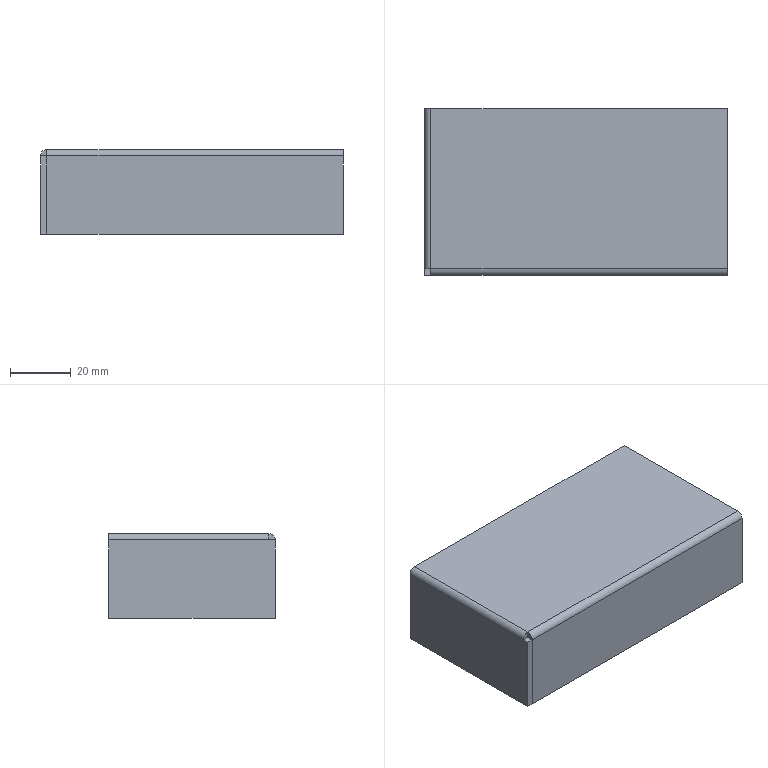Part | STEP file | 1 solid | 23 faces | box 100 x 55 x 28 mm | volume 18799 mm3 | plane 19 | cylinder 4 | commonest cylinder face diameters 0.2 x2 4.2 x2
STEP:
#1=CARTESIAN_POINT('',(0.,0.,0.));
#2=DIRECTION('',(0.,0.,1.));
#3=DIRECTION('',(1.,0.,0.));
#4=AXIS2_PLACEMENT_3D('',#1,#2,#3);
#5=CARTESIAN_POINT('',(-50.,-25.4,-2.1));
#6=VERTEX_POINT('',#5);
#7=CARTESIAN_POINT('',(-48.,-25.4,-2.1));
#8=VERTEX_POINT('',#7);
#9=CARTESIAN_POINT('',(-50.,-25.4,-2.1));
#10=DIRECTION('',(1.,0.,0.));
#11=VECTOR('',#10,1.);
#12=LINE('',#9,#11);
#13=CARTESIAN_POINT('',(0.,0.,-2.1));
#14=DIRECTION('',(0.,0.,1.));
#15=DIRECTION('',(1.,0.,0.));
#16=AXIS2_PLACEMENT_3D('',#13,#14,#15);
#17=PLANE('',#16);
#18=CARTESIAN_POINT('',(-50.,-25.4));
#19=DIRECTION('',(1.,0.));
#20=VECTOR('',#19,1.);
#21=LINE('',#18,#20);
#22=(GEOMETRIC_REPRESENTATION_CONTEXT(2)PARAMETRIC_REPRESENTATION_CONTEXT()REPRESENTATION_CONTEXT('',''));
#23=DEFINITIONAL_REPRESENTATION('',(#21),#22);
#24=PCURVE('',#17,#23);
#25=CARTESIAN_POINT('',(-47.9,-25.4,-2.1));
#26=DIRECTION('',(0.,-1.,0.));
#27=DIRECTION('',(0.,0.,-1.));
#28=AXIS2_PLACEMENT_3D('',#25,#26,#27);
#29=PLANE('',#28);
#30=CARTESIAN_POINT('',(0.,-2.1));
#31=DIRECTION('',(0.,1.));
#32=VECTOR('',#31,1.);
#33=LINE('',#30,#32);
#34=(GEOMETRIC_REPRESENTATION_CONTEXT(2)PARAMETRIC_REPRESENTATION_CONTEXT()REPRESENTATION_CONTEXT('',''));
#35=DEFINITIONAL_REPRESENTATION('',(#33),#34);
#36=PCURVE('',#29,#35);
#37=SURFACE_CURVE('',#12,(#24,#36),.PCURVE_S1.);
#38=EDGE_CURVE('',#6,#8,#37,.T.);
#39=ORIENTED_EDGE('',*,*,#38,.F.);
#40=CARTESIAN_POINT('',(-50.,-27.5,-2.1));
#41=VERTEX_POINT('',#40);
#42=CARTESIAN_POINT('',(-50.,-27.5,-2.1));
#43=DIRECTION('',(0.,-1.,0.));
#44=VECTOR('',#43,1.);
#45=LINE('',#42,#44);
#46=CARTESIAN_POINT('',(-50.,-27.5));
#47=DIRECTION('',(0.,-1.));
#48=VECTOR('',#47,1.);
#49=LINE('',#46,#48);
#50=(GEOMETRIC_REPRESENTATION_CONTEXT(2)PARAMETRIC_REPRESENTATION_CONTEXT()REPRESENTATION_CONTEXT('',''));
#51=DEFINITIONAL_REPRESENTATION('',(#49),#50);
#52=PCURVE('',#17,#51);
#53=CARTESIAN_POINT('',(-50.,0.,0.));
#54=DIRECTION('',(1.,0.,0.));
#55=DIRECTION('',(0.,0.,-1.));
#56=AXIS2_PLACEMENT_3D('',#53,#54,#55);
#57=PLANE('',#56);
#58=CARTESIAN_POINT('',(2.1,-27.5));
#59=DIRECTION('',(0.,-1.));
#60=VECTOR('',#59,1.);
#61=LINE('',#58,#60);
#62=(GEOMETRIC_REPRESENTATION_CONTEXT(2)PARAMETRIC_REPRESENTATION_CONTEXT()REPRESENTATION_CONTEXT('',''));
#63=DEFINITIONAL_REPRESENTATION('',(#61),#62);
#64=PCURVE('',#57,#63);
#65=SURFACE_CURVE('',#45,(#52,#64),.PCURVE_S1.);
#66=EDGE_CURVE('',#6,#41,#65,.T.);
#67=ORIENTED_EDGE('',*,*,#66,.T.);
#68=CARTESIAN_POINT('',(-48.,-27.5,-2.1));
#69=VERTEX_POINT('',#68);
#70=CARTESIAN_POINT('',(-50.,-27.5,-2.1));
#71=DIRECTION('',(-1.,0.,0.));
#72=VECTOR('',#71,1.);
#73=LINE('',#70,#72);
#74=CARTESIAN_POINT('',(-50.,-27.5));
#75=DIRECTION('',(-1.,0.));
#76=VECTOR('',#75,1.);
#77=LINE('',#74,#76);
#78=(GEOMETRIC_REPRESENTATION_CONTEXT(2)PARAMETRIC_REPRESENTATION_CONTEXT()REPRESENTATION_CONTEXT('',''));
#79=DEFINITIONAL_REPRESENTATION('',(#77),#78);
#80=PCURVE('',#17,#79);
#81=CARTESIAN_POINT('',(-50.,-27.5,-2.));
#82=DIRECTION('',(0.,1.,0.));
#83=DIRECTION('',(-1.,0.,0.));
#84=AXIS2_PLACEMENT_3D('',#81,#82,#83);
#85=PLANE('',#84);
#86=CARTESIAN_POINT('',(0.,-0.1));
#87=DIRECTION('',(1.,0.));
#88=VECTOR('',#87,1.);
#89=LINE('',#86,#88);
#90=(GEOMETRIC_REPRESENTATION_CONTEXT(2)PARAMETRIC_REPRESENTATION_CONTEXT()REPRESENTATION_CONTEXT('',''));
#91=DEFINITIONAL_REPRESENTATION('',(#89),#90);
#92=PCURVE('',#85,#91);
#93=SURFACE_CURVE('',#73,(#80,#92),.PCURVE_S1.);
#94=EDGE_CURVE('',#69,#41,#93,.T.);
#95=ORIENTED_EDGE('',*,*,#94,.F.);
#96=CARTESIAN_POINT('',(-48.,-27.5,-2.1));
#97=DIRECTION('',(0.,1.,0.));
#98=VECTOR('',#97,1.);
#99=LINE('',#96,#98);
#100=CARTESIAN_POINT('',(-48.,-27.5));
#101=DIRECTION('',(0.,1.));
#102=VECTOR('',#101,1.);
#103=LINE('',#100,#102);
#104=(GEOMETRIC_REPRESENTATION_CONTEXT(2)PARAMETRIC_REPRESENTATION_CONTEXT()REPRESENTATION_CONTEXT('',''));
#105=DEFINITIONAL_REPRESENTATION('',(#103),#104);
#106=PCURVE('',#17,#105);
#107=CARTESIAN_POINT('',(-48.,0.,0.));
#108=DIRECTION('',(1.,0.,0.));
#109=DIRECTION('',(0.,0.,-1.));
#110=AXIS2_PLACEMENT_3D('',#107,#108,#109);
#111=PLANE('',#110);
#112=CARTESIAN_POINT('',(2.1,-27.5));
#113=DIRECTION('',(0.,1.));
#114=VECTOR('',#113,1.);
#115=LINE('',#112,#114);
#116=(GEOMETRIC_REPRESENTATION_CONTEXT(2)PARAMETRIC_REPRESENTATION_CONTEXT()REPRESENTATION_CONTEXT('',''));
#117=DEFINITIONAL_REPRESENTATION('',(#115),#116);
#118=PCURVE('',#111,#117);
#119=SURFACE_CURVE('',#99,(#106,#118),.PCURVE_S1.);
#120=EDGE_CURVE('',#69,#8,#119,.T.);
#121=ORIENTED_EDGE('',*,*,#120,.T.);
#122=EDGE_LOOP('',(#39,#67,#95,#121));
#123=FACE_BOUND('',#122,.T.);
#124=ADVANCED_FACE('',(#123),#17,.T.);
#125=CARTESIAN_POINT('',(-50.,27.5,-2.1));
#126=VERTEX_POINT('',#125);
#127=CARTESIAN_POINT('',(-50.,-27.5,-2.1));
#128=DIRECTION('',(0.,-1.,0.));
#129=VECTOR('',#128,1.);
#130=LINE('',#127,#129);
#131=CARTESIAN_POINT('',(-47.9,27.5,-2.1));
#132=DIRECTION('',(0.,1.,0.));
#133=DIRECTION('',(-1.,0.,0.));
#134=AXIS2_PLACEMENT_3D('',#131,#132,#133);
#135=CYLINDRICAL_SURFACE('',#134,2.1);
#136=CARTESIAN_POINT('',(0.,0.));
#137=CARTESIAN_POINT('',(0.,-0.8015));
#138=CARTESIAN_POINT('',(0.,-2.405));
#139=CARTESIAN_POINT('',(0.,-4.809));
#140=CARTESIAN_POINT('',(0.,-7.214));
#141=CARTESIAN_POINT('',(0.,-9.618));
#142=CARTESIAN_POINT('',(0.,-12.023));
#143=CARTESIAN_POINT('',(0.,-14.427));
#144=CARTESIAN_POINT('',(0.,-16.832));
#145=CARTESIAN_POINT('',(0.,-19.236));
#146=CARTESIAN_POINT('',(0.,-21.641));
#147=CARTESIAN_POINT('',(0.,-24.045));
#148=CARTESIAN_POINT('',(0.,-26.45));
#149=CARTESIAN_POINT('',(0.,-28.855));
#150=CARTESIAN_POINT('',(0.,-31.259));
#151=CARTESIAN_POINT('',(0.,-33.664));
#152=CARTESIAN_POINT('',(0.,-36.068));
#153=CARTESIAN_POINT('',(0.,-38.473));
#154=CARTESIAN_POINT('',(0.,-40.877));
#155=CARTESIAN_POINT('',(0.,-43.282));
#156=CARTESIAN_POINT('',(0.,-45.686));
#157=CARTESIAN_POINT('',(0.,-48.091));
#158=CARTESIAN_POINT('',(0.,-50.495));
#159=CARTESIAN_POINT('',(0.,-52.098));
#160=CARTESIAN_POINT('',(0.,-52.9));
#161=B_SPLINE_CURVE_WITH_KNOTS('',3,(#136,#137,#138,#139,#140,#141,#142,#143,#144,#145,#146,#147,#148,#149,#150,#151,#152,#153,#154,#155,#156,#157,#158,#159,#160),.UNSPECIFIED.,.F.,.F.,(4,1,1,1,1,1,1,1,1,1,1,1,1,1,1,1,1,1,1,1,1,1,4),(-55.,-52.595,-50.191,-47.786,-45.382,-42.977,-40.573,-38.168,-35.764,-33.359,-30.955,-28.55,-26.145,-23.741,-21.336,-18.932,-16.527,-14.123,-11.718,-9.314,-6.909,-4.505,-2.1),.QUASI_UNIFORM_KNOTS.);
#162=(GEOMETRIC_REPRESENTATION_CONTEXT(2)PARAMETRIC_REPRESENTATION_CONTEXT()REPRESENTATION_CONTEXT('',''));
#163=DEFINITIONAL_REPRESENTATION('',(#161),#162);
#164=PCURVE('',#135,#163);
#165=CARTESIAN_POINT('',(2.1,-27.5));
#166=DIRECTION('',(0.,-1.));
#167=VECTOR('',#166,1.);
#168=LINE('',#165,#167);
#169=(GEOMETRIC_REPRESENTATION_CONTEXT(2)PARAMETRIC_REPRESENTATION_CONTEXT()REPRESENTATION_CONTEXT('',''));
#170=DEFINITIONAL_REPRESENTATION('',(#168),#169);
#171=PCURVE('',#57,#170);
#172=SURFACE_CURVE('',#130,(#164,#171),.PCURVE_S1.);
#173=EDGE_CURVE('',#126,#6,#172,.T.);
#174=ORIENTED_EDGE('',*,*,#173,.T.);
#175=CARTESIAN_POINT('',(-47.9,-25.4,0.));
#176=VERTEX_POINT('',#175);
#177=CARTESIAN_POINT('',(-47.9,-25.4,-2.1));
#178=DIRECTION('',(0.,1.,0.));
#179=DIRECTION('',(0.,0.,-1.));
#180=AXIS2_PLACEMENT_3D('',#177,#178,#179);
#181=CIRCLE('',#180,2.1);
#182=CARTESIAN_POINT('',(-1.571,-52.9));
#183=DIRECTION('',(1.,0.));
#184=VECTOR('',#183,1.);
#185=LINE('',#182,#184);
#186=(GEOMETRIC_REPRESENTATION_CONTEXT(2)PARAMETRIC_REPRESENTATION_CONTEXT()REPRESENTATION_CONTEXT('',''));
#187=DEFINITIONAL_REPRESENTATION('',(#185),#186);
#188=PCURVE('',#135,#187);
#189=CARTESIAN_POINT('',(2.1,0.));
#190=CARTESIAN_POINT('',(2.1,-3.637));
#191=CARTESIAN_POINT('',(-1.05,-1.819));
#192=CARTESIAN_POINT('',(-4.2,0.));
#193=CARTESIAN_POINT('',(-1.05,1.819));
#194=CARTESIAN_POINT('',(2.1,3.637));
#195=CARTESIAN_POINT('',(2.1,0.));
#196=(BOUNDED_CURVE()B_SPLINE_CURVE(2,(#189,#190,#191,#192,#193,#194,#195),.UNSPECIFIED.,.T.,.F.)B_SPLINE_CURVE_WITH_KNOTS((1,2,2,2,2,1),(-2.094,0.,2.094,4.189,6.283,8.378),.UNSPECIFIED.)CURVE()GEOMETRIC_REPRESENTATION_ITEM()RATIONAL_B_SPLINE_CURVE((1.,0.5,1.,0.5,1.,0.5,1.))REPRESENTATION_ITEM(''));
#197=(GEOMETRIC_REPRESENTATION_CONTEXT(2)PARAMETRIC_REPRESENTATION_CONTEXT()REPRESENTATION_CONTEXT('',''));
#198=DEFINITIONAL_REPRESENTATION('',(#196),#197);
#199=PCURVE('',#29,#198);
#200=SURFACE_CURVE('',#181,(#188,#199),.PCURVE_S1.);
#201=EDGE_CURVE('',#6,#176,#200,.T.);
#202=ORIENTED_EDGE('',*,*,#201,.T.);
#203=CARTESIAN_POINT('',(-47.9,27.5,0.));
#204=VERTEX_POINT('',#203);
#205=CARTESIAN_POINT('',(-47.9,27.5,0.));
#206=DIRECTION('',(0.,-1.,0.));
#207=VECTOR('',#206,1.);
#208=LINE('',#205,#207);
#209=CARTESIAN_POINT('',(1.571,0.));
#210=DIRECTION('',(0.,-1.));
#211=VECTOR('',#210,1.);
#212=LINE('',#209,#211);
#213=(GEOMETRIC_REPRESENTATION_CONTEXT(2)PARAMETRIC_REPRESENTATION_CONTEXT()REPRESENTATION_CONTEXT('',''));
#214=DEFINITIONAL_REPRESENTATION('',(#212),#213);
#215=PCURVE('',#135,#214);
#216=CARTESIAN_POINT('',(0.,0.,0.));
#217=DIRECTION('',(0.,0.,1.));
#218=DIRECTION('',(1.,0.,0.));
#219=AXIS2_PLACEMENT_3D('',#216,#217,#218);
#220=PLANE('',#219);
#221=CARTESIAN_POINT('',(-47.9,27.5));
#222=DIRECTION('',(0.,-1.));
#223=VECTOR('',#222,1.);
#224=LINE('',#221,#223);
#225=(GEOMETRIC_REPRESENTATION_CONTEXT(2)PARAMETRIC_REPRESENTATION_CONTEXT()REPRESENTATION_CONTEXT('',''));
#226=DEFINITIONAL_REPRESENTATION('',(#224),#225);
#227=PCURVE('',#220,#226);
#228=SURFACE_CURVE('',#208,(#215,#227),.PCURVE_S1.);
#229=EDGE_CURVE('',#204,#176,#228,.T.);
#230=ORIENTED_EDGE('',*,*,#229,.F.);
#231=CARTESIAN_POINT('',(-47.9,27.5,-2.1));
#232=DIRECTION('',(0.,1.,0.));
#233=DIRECTION('',(0.,0.,1.));
#234=AXIS2_PLACEMENT_3D('',#231,#232,#233);
#235=CIRCLE('',#234,2.1);
#236=CARTESIAN_POINT('',(-4.712,0.));
#237=DIRECTION('',(1.,0.));
#238=VECTOR('',#237,1.);
#239=LINE('',#236,#238);
#240=(GEOMETRIC_REPRESENTATION_CONTEXT(2)PARAMETRIC_REPRESENTATION_CONTEXT()REPRESENTATION_CONTEXT('',''));
#241=DEFINITIONAL_REPRESENTATION('',(#239),#240);
#242=PCURVE('',#135,#241);
#243=CARTESIAN_POINT('',(-47.9,27.5,-2.1));
#244=DIRECTION('',(0.,-1.,0.));
#245=DIRECTION('',(0.,0.,-1.));
#246=AXIS2_PLACEMENT_3D('',#243,#244,#245);
#247=PLANE('',#246);
#248=CARTESIAN_POINT('',(-2.1,0.));
#249=CARTESIAN_POINT('',(-2.1,3.637));
#250=CARTESIAN_POINT('',(1.05,1.819));
#251=CARTESIAN_POINT('',(4.2,0.));
#252=CARTESIAN_POINT('',(1.05,-1.819));
#253=CARTESIAN_POINT('',(-2.1,-3.637));
#254=CARTESIAN_POINT('',(-2.1,0.));
#255=(BOUNDED_CURVE()B_SPLINE_CURVE(2,(#248,#249,#250,#251,#252,#253,#254),.UNSPECIFIED.,.T.,.F.)B_SPLINE_CURVE_WITH_KNOTS((1,2,2,2,2,1),(-2.094,0.,2.094,4.189,6.283,8.378),.UNSPECIFIED.)CURVE()GEOMETRIC_REPRESENTATION_ITEM()RATIONAL_B_SPLINE_CURVE((1.,0.5,1.,0.5,1.,0.5,1.))REPRESENTATION_ITEM(''));
#256=(GEOMETRIC_REPRESENTATION_CONTEXT(2)PARAMETRIC_REPRESENTATION_CONTEXT()REPRESENTATION_CONTEXT('',''));
#257=DEFINITIONAL_REPRESENTATION('',(#255),#256);
#258=PCURVE('',#247,#257);
#259=SURFACE_CURVE('',#235,(#242,#258),.PCURVE_S1.);
#260=EDGE_CURVE('',#126,#204,#259,.T.);
#261=ORIENTED_EDGE('',*,*,#260,.F.);
#262=EDGE_LOOP('',(#174,#202,#230,#261));
#263=FACE_BOUND('',#262,.T.);
#264=ADVANCED_FACE('',(#263),#135,.T.);
#265=CARTESIAN_POINT('',(-47.9,-25.4,-2.));
#266=VERTEX_POINT('',#265);
#267=CARTESIAN_POINT('',(50.,-25.4,-2.));
#268=VERTEX_POINT('',#267);
#269=CARTESIAN_POINT('',(-47.9,-25.4,-2.));
#270=DIRECTION('',(1.,0.,0.));
#271=VECTOR('',#270,1.);
#272=LINE('',#269,#271);
#273=CARTESIAN_POINT('',(0.,0.,-2.));
#274=DIRECTION('',(0.,0.,1.));
#275=DIRECTION('',(1.,0.,0.));
#276=AXIS2_PLACEMENT_3D('',#273,#274,#275);
#277=PLANE('',#276);
#278=CARTESIAN_POINT('',(-47.9,-25.4));
#279=DIRECTION('',(1.,0.));
#280=VECTOR('',#279,1.);
#281=LINE('',#278,#280);
#282=(GEOMETRIC_REPRESENTATION_CONTEXT(2)PARAMETRIC_REPRESENTATION_CONTEXT()REPRESENTATION_CONTEXT('',''));
#283=DEFINITIONAL_REPRESENTATION('',(#281),#282);
#284=PCURVE('',#277,#283);
#285=CARTESIAN_POINT('',(-47.9,-25.4,-2.1));
#286=DIRECTION('',(-1.,0.,0.));
#287=DIRECTION('',(0.,-1.,0.));
#288=AXIS2_PLACEMENT_3D('',#285,#286,#287);
#289=CYLINDRICAL_SURFACE('',#288,0.1);
#290=CARTESIAN_POINT('',(1.571,0.));
#291=DIRECTION('',(0.,-1.));
#292=VECTOR('',#291,1.);
#293=LINE('',#290,#292);
#294=(GEOMETRIC_REPRESENTATION_CONTEXT(2)PARAMETRIC_REPRESENTATION_CONTEXT()REPRESENTATION_CONTEXT('',''));
#295=DEFINITIONAL_REPRESENTATION('',(#293),#294);
#296=PCURVE('',#289,#295);
#297=SURFACE_CURVE('',#272,(#284,#296),.PCURVE_S1.);
#298=EDGE_CURVE('',#266,#268,#297,.T.);
#299=ORIENTED_EDGE('',*,*,#298,.F.);
#300=CARTESIAN_POINT('',(-47.9,27.5,-2.));
#301=VERTEX_POINT('',#300);
#302=CARTESIAN_POINT('',(-47.9,27.5,-2.));
#303=DIRECTION('',(0.,-1.,0.));
#304=VECTOR('',#303,1.);
#305=LINE('',#302,#304);
#306=CARTESIAN_POINT('',(-47.9,27.5));
#307=DIRECTION('',(0.,-1.));
#308=VECTOR('',#307,1.);
#309=LINE('',#306,#308);
#310=(GEOMETRIC_REPRESENTATION_CONTEXT(2)PARAMETRIC_REPRESENTATION_CONTEXT()REPRESENTATION_CONTEXT('',''));
#311=DEFINITIONAL_REPRESENTATION('',(#309),#310);
#312=PCURVE('',#277,#311);
#313=CARTESIAN_POINT('',(-47.9,27.5,-2.1));
#314=DIRECTION('',(0.,1.,0.));
#315=DIRECTION('',(-1.,0.,0.));
#316=AXIS2_PLACEMENT_3D('',#313,#314,#315);
#317=CYLINDRICAL_SURFACE('',#316,0.1);
#318=CARTESIAN_POINT('',(1.571,0.));
#319=DIRECTION('',(0.,-1.));
#320=VECTOR('',#319,1.);
#321=LINE('',#318,#320);
#322=(GEOMETRIC_REPRESENTATION_CONTEXT(2)PARAMETRIC_REPRESENTATION_CONTEXT()REPRESENTATION_CONTEXT('',''));
#323=DEFINITIONAL_REPRESENTATION('',(#321),#322);
#324=PCURVE('',#317,#323);
#325=SURFACE_CURVE('',#305,(#312,#324),.PCURVE_S1.);
#326=EDGE_CURVE('',#301,#266,#325,.T.);
#327=ORIENTED_EDGE('',*,*,#326,.F.);
#328=CARTESIAN_POINT('',(50.,27.5,-2.));
#329=VERTEX_POINT('',#328);
#330=CARTESIAN_POINT('',(-50.,27.5,-2.));
#331=DIRECTION('',(-1.,0.,0.));
#332=VECTOR('',#331,1.);
#333=LINE('',#330,#332);
#334=CARTESIAN_POINT('',(-50.,27.5));
#335=DIRECTION('',(-1.,0.));
#336=VECTOR('',#335,1.);
#337=LINE('',#334,#336);
#338=(GEOMETRIC_REPRESENTATION_CONTEXT(2)PARAMETRIC_REPRESENTATION_CONTEXT()REPRESENTATION_CONTEXT('',''));
#339=DEFINITIONAL_REPRESENTATION('',(#337),#338);
#340=PCURVE('',#277,#339);
#341=CARTESIAN_POINT('',(-50.,27.5,-2.));
#342=DIRECTION('',(0.,1.,0.));
#343=DIRECTION('',(0.,0.,1.));
#344=AXIS2_PLACEMENT_3D('',#341,#342,#343);
#345=PLANE('',#344);
#346=CARTESIAN_POINT('',(0.,0.));
#347=DIRECTION('',(0.,-1.));
#348=VECTOR('',#347,1.);
#349=LINE('',#346,#348);
#350=(GEOMETRIC_REPRESENTATION_CONTEXT(2)PARAMETRIC_REPRESENTATION_CONTEXT()REPRESENTATION_CONTEXT('',''));
#351=DEFINITIONAL_REPRESENTATION('',(#349),#350);
#352=PCURVE('',#345,#351);
#353=SURFACE_CURVE('',#333,(#340,#352),.PCURVE_S1.);
#354=EDGE_CURVE('',#329,#301,#353,.T.);
#355=ORIENTED_EDGE('',*,*,#354,.F.);
#356=CARTESIAN_POINT('',(50.,27.5,-2.));
#357=DIRECTION('',(0.,1.,0.));
#358=VECTOR('',#357,1.);
#359=LINE('',#356,#358);
#360=CARTESIAN_POINT('',(50.,27.5));
#361=DIRECTION('',(0.,1.));
#362=VECTOR('',#361,1.);
#363=LINE('',#360,#362);
#364=(GEOMETRIC_REPRESENTATION_CONTEXT(2)PARAMETRIC_REPRESENTATION_CONTEXT()REPRESENTATION_CONTEXT('',''));
#365=DEFINITIONAL_REPRESENTATION('',(#363),#364);
#366=PCURVE('',#277,#365);
#367=CARTESIAN_POINT('',(50.,27.5,-2.));
#368=DIRECTION('',(1.,0.,0.));
#369=DIRECTION('',(0.,0.,-1.));
#370=AXIS2_PLACEMENT_3D('',#367,#368,#369);
#371=PLANE('',#370);
#372=CARTESIAN_POINT('',(0.,0.));
#373=DIRECTION('',(0.,1.));
#374=VECTOR('',#373,1.);
#375=LINE('',#372,#374);
#376=(GEOMETRIC_REPRESENTATION_CONTEXT(2)PARAMETRIC_REPRESENTATION_CONTEXT()REPRESENTATION_CONTEXT('',''));
#377=DEFINITIONAL_REPRESENTATION('',(#375),#376);
#378=PCURVE('',#371,#377);
#379=SURFACE_CURVE('',#359,(#366,#378),.PCURVE_S1.);
#380=EDGE_CURVE('',#268,#329,#379,.T.);
#381=ORIENTED_EDGE('',*,*,#380,.F.);
#382=EDGE_LOOP('',(#299,#327,#355,#381));
#383=FACE_BOUND('',#382,.T.);
#384=ADVANCED_FACE('',(#383),#277,.F.);
#385=ORIENTED_EDGE('',*,*,#229,.T.);
#386=CARTESIAN_POINT('',(50.,-25.4,0.));
#387=VERTEX_POINT('',#386);
#388=CARTESIAN_POINT('',(-47.9,-25.4,0.));
#389=DIRECTION('',(1.,0.,0.));
#390=VECTOR('',#389,1.);
#391=LINE('',#388,#390);
#392=CARTESIAN_POINT('',(-47.9,-25.4));
#393=DIRECTION('',(1.,0.));
#394=VECTOR('',#393,1.);
#395=LINE('',#392,#394);
#396=(GEOMETRIC_REPRESENTATION_CONTEXT(2)PARAMETRIC_REPRESENTATION_CONTEXT()REPRESENTATION_CONTEXT('',''));
#397=DEFINITIONAL_REPRESENTATION('',(#395),#396);
#398=PCURVE('',#220,#397);
#399=CARTESIAN_POINT('',(-47.9,-25.4,-2.1));
#400=DIRECTION('',(-1.,0.,0.));
#401=DIRECTION('',(0.,-1.,0.));
#402=AXIS2_PLACEMENT_3D('',#399,#400,#401);
#403=CYLINDRICAL_SURFACE('',#402,2.1);
#404=CARTESIAN_POINT('',(1.571,0.));
#405=DIRECTION('',(0.,-1.));
#406=VECTOR('',#405,1.);
#407=LINE('',#404,#406);
#408=(GEOMETRIC_REPRESENTATION_CONTEXT(2)PARAMETRIC_REPRESENTATION_CONTEXT()REPRESENTATION_CONTEXT('',''));
#409=DEFINITIONAL_REPRESENTATION('',(#407),#408);
#410=PCURVE('',#403,#409);
#411=SURFACE_CURVE('',#391,(#398,#410),.PCURVE_S1.);
#412=EDGE_CURVE('',#176,#387,#411,.T.);
#413=ORIENTED_EDGE('',*,*,#412,.T.);
#414=CARTESIAN_POINT('',(50.,27.5,0.));
#415=VERTEX_POINT('',#414);
#416=CARTESIAN_POINT('',(50.,27.5,0.));
#417=DIRECTION('',(0.,1.,0.));
#418=VECTOR('',#417,1.);
#419=LINE('',#416,#418);
#420=CARTESIAN_POINT('',(50.,27.5));
#421=DIRECTION('',(0.,1.));
#422=VECTOR('',#421,1.);
#423=LINE('',#420,#422);
#424=(GEOMETRIC_REPRESENTATION_CONTEXT(2)PARAMETRIC_REPRESENTATION_CONTEXT()REPRESENTATION_CONTEXT('',''));
#425=DEFINITIONAL_REPRESENTATION('',(#423),#424);
#426=PCURVE('',#220,#425);
#427=CARTESIAN_POINT('',(-2.,0.));
#428=DIRECTION('',(0.,1.));
#429=VECTOR('',#428,1.);
#430=LINE('',#427,#429);
#431=(GEOMETRIC_REPRESENTATION_CONTEXT(2)PARAMETRIC_REPRESENTATION_CONTEXT()REPRESENTATION_CONTEXT('',''));
#432=DEFINITIONAL_REPRESENTATION('',(#430),#431);
#433=PCURVE('',#371,#432);
#434=SURFACE_CURVE('',#419,(#426,#433),.PCURVE_S1.);
#435=EDGE_CURVE('',#387,#415,#434,.T.);
#436=ORIENTED_EDGE('',*,*,#435,.T.);
#437=CARTESIAN_POINT('',(-50.,27.5,0.));
#438=DIRECTION('',(-1.,0.,0.));
#439=VECTOR('',#438,1.);
#440=LINE('',#437,#439);
#441=CARTESIAN_POINT('',(-50.,27.5));
#442=DIRECTION('',(-1.,0.));
#443=VECTOR('',#442,1.);
#444=LINE('',#441,#443);
#445=(GEOMETRIC_REPRESENTATION_CONTEXT(2)PARAMETRIC_REPRESENTATION_CONTEXT()REPRESENTATION_CONTEXT('',''));
#446=DEFINITIONAL_REPRESENTATION('',(#444),#445);
#447=PCURVE('',#220,#446);
#448=CARTESIAN_POINT('',(2.,0.));
#449=DIRECTION('',(0.,-1.));
#450=VECTOR('',#449,1.);
#451=LINE('',#448,#450);
#452=(GEOMETRIC_REPRESENTATION_CONTEXT(2)PARAMETRIC_REPRESENTATION_CONTEXT()REPRESENTATION_CONTEXT('',''));
#453=DEFINITIONAL_REPRESENTATION('',(#451),#452);
#454=PCURVE('',#345,#453);
#455=SURFACE_CURVE('',#440,(#447,#454),.PCURVE_S1.);
#456=EDGE_CURVE('',#415,#204,#455,.T.);
#457=ORIENTED_EDGE('',*,*,#456,.T.);
#458=EDGE_LOOP('',(#385,#413,#436,#457));
#459=FACE_BOUND('',#458,.T.);
#460=ADVANCED_FACE('',(#459),#220,.T.);
#461=ORIENTED_EDGE('',*,*,#354,.T.);
#462=CARTESIAN_POINT('',(-47.9,27.5,-2.));
#463=DIRECTION('',(0.,0.,1.));
#464=VECTOR('',#463,1.);
#465=LINE('',#462,#464);
#466=CARTESIAN_POINT('',(0.,2.1));
#467=DIRECTION('',(1.,0.));
#468=VECTOR('',#467,1.);
#469=LINE('',#466,#468);
#470=(GEOMETRIC_REPRESENTATION_CONTEXT(2)PARAMETRIC_REPRESENTATION_CONTEXT()REPRESENTATION_CONTEXT('',''));
#471=DEFINITIONAL_REPRESENTATION('',(#469),#470);
#472=PCURVE('',#345,#471);
#473=CARTESIAN_POINT('',(-0.1,0.));
#474=DIRECTION('',(-1.,0.));
#475=VECTOR('',#474,1.);
#476=LINE('',#473,#475);
#477=(GEOMETRIC_REPRESENTATION_CONTEXT(2)PARAMETRIC_REPRESENTATION_CONTEXT()REPRESENTATION_CONTEXT('',''));
#478=DEFINITIONAL_REPRESENTATION('',(#476),#477);
#479=PCURVE('',#247,#478);
#480=SURFACE_CURVE('',#465,(#472,#479),.PCURVE_S1.);
#481=EDGE_CURVE('',#301,#204,#480,.T.);
#482=ORIENTED_EDGE('',*,*,#481,.T.);
#483=ORIENTED_EDGE('',*,*,#456,.F.);
#484=CARTESIAN_POINT('',(50.,27.5,-2.));
#485=DIRECTION('',(0.,0.,1.));
#486=VECTOR('',#485,1.);
#487=LINE('',#484,#486);
#488=CARTESIAN_POINT('',(0.,100.));
#489=DIRECTION('',(1.,0.));
#490=VECTOR('',#489,1.);
#491=LINE('',#488,#490);
#492=(GEOMETRIC_REPRESENTATION_CONTEXT(2)PARAMETRIC_REPRESENTATION_CONTEXT()REPRESENTATION_CONTEXT('',''));
#493=DEFINITIONAL_REPRESENTATION('',(#491),#492);
#494=PCURVE('',#345,#493);
#495=CARTESIAN_POINT('',(0.,0.));
#496=DIRECTION('',(-1.,0.));
#497=VECTOR('',#496,1.);
#498=LINE('',#495,#497);
#499=(GEOMETRIC_REPRESENTATION_CONTEXT(2)PARAMETRIC_REPRESENTATION_CONTEXT()REPRESENTATION_CONTEXT('',''));
#500=DEFINITIONAL_REPRESENTATION('',(#498),#499);
#501=PCURVE('',#371,#500);
#502=SURFACE_CURVE('',#487,(#494,#501),.PCURVE_S1.);
#503=EDGE_CURVE('',#329,#415,#502,.T.);
#504=ORIENTED_EDGE('',*,*,#503,.F.);
#505=EDGE_LOOP('',(#461,#482,#483,#504));
#506=FACE_BOUND('',#505,.T.);
#507=ADVANCED_FACE('',(#506),#345,.T.);
#508=CARTESIAN_POINT('',(50.,-25.4,-2.));
#509=DIRECTION('',(0.,0.,1.));
#510=VECTOR('',#509,1.);
#511=LINE('',#508,#510);
#512=CARTESIAN_POINT('',(0.,-52.9));
#513=DIRECTION('',(-1.,0.));
#514=VECTOR('',#513,1.);
#515=LINE('',#512,#514);
#516=(GEOMETRIC_REPRESENTATION_CONTEXT(2)PARAMETRIC_REPRESENTATION_CONTEXT()REPRESENTATION_CONTEXT('',''));
#517=DEFINITIONAL_REPRESENTATION('',(#515),#516);
#518=PCURVE('',#371,#517);
#519=CARTESIAN_POINT('',(50.,-25.4,-2.1));
#520=DIRECTION('',(1.,0.,0.));
#521=DIRECTION('',(0.,0.,-1.));
#522=AXIS2_PLACEMENT_3D('',#519,#520,#521);
#523=PLANE('',#522);
#524=CARTESIAN_POINT('',(-0.1,0.));
#525=DIRECTION('',(-1.,0.));
#526=VECTOR('',#525,1.);
#527=LINE('',#524,#526);
#528=(GEOMETRIC_REPRESENTATION_CONTEXT(2)PARAMETRIC_REPRESENTATION_CONTEXT()REPRESENTATION_CONTEXT('',''));
#529=DEFINITIONAL_REPRESENTATION('',(#527),#528);
#530=PCURVE('',#523,#529);
#531=SURFACE_CURVE('',#511,(#518,#530),.PCURVE_S1.);
#532=EDGE_CURVE('',#268,#387,#531,.T.);
#533=ORIENTED_EDGE('',*,*,#532,.F.);
#534=ORIENTED_EDGE('',*,*,#380,.T.);
#535=ORIENTED_EDGE('',*,*,#503,.T.);
#536=ORIENTED_EDGE('',*,*,#435,.F.);
#537=EDGE_LOOP('',(#533,#534,#535,#536));
#538=FACE_BOUND('',#537,.T.);
#539=ADVANCED_FACE('',(#538),#371,.T.);
#540=CARTESIAN_POINT('',(-48.,27.5,-2.1));
#541=VERTEX_POINT('',#540);
#542=CARTESIAN_POINT('',(-47.9,27.5,-2.1));
#543=DIRECTION('',(0.,1.,0.));
#544=DIRECTION('',(0.,0.,1.));
#545=AXIS2_PLACEMENT_3D('',#542,#543,#544);
#546=CIRCLE('',#545,0.1);
#547=CARTESIAN_POINT('',(-0.1,0.));
#548=CARTESIAN_POINT('',(-0.1,0.1732));
#549=CARTESIAN_POINT('',(0.05,0.0866));
#550=CARTESIAN_POINT('',(0.2,0.));
#551=CARTESIAN_POINT('',(0.05,-0.0866));
#552=CARTESIAN_POINT('',(-0.1,-0.1732));
#553=CARTESIAN_POINT('',(-0.1,0.));
#554=(BOUNDED_CURVE()B_SPLINE_CURVE(2,(#547,#548,#549,#550,#551,#552,#553),.UNSPECIFIED.,.T.,.F.)B_SPLINE_CURVE_WITH_KNOTS((1,2,2,2,2,1),(-2.094,0.,2.094,4.189,6.283,8.378),.UNSPECIFIED.)CURVE()GEOMETRIC_REPRESENTATION_ITEM()RATIONAL_B_SPLINE_CURVE((1.,0.5,1.,0.5,1.,0.5,1.))REPRESENTATION_ITEM(''));
#555=(GEOMETRIC_REPRESENTATION_CONTEXT(2)PARAMETRIC_REPRESENTATION_CONTEXT()REPRESENTATION_CONTEXT('',''));
#556=DEFINITIONAL_REPRESENTATION('',(#554),#555);
#557=PCURVE('',#247,#556);
#558=CARTESIAN_POINT('',(-4.712,0.));
#559=DIRECTION('',(1.,0.));
#560=VECTOR('',#559,1.);
#561=LINE('',#558,#560);
#562=(GEOMETRIC_REPRESENTATION_CONTEXT(2)PARAMETRIC_REPRESENTATION_CONTEXT()REPRESENTATION_CONTEXT('',''));
#563=DEFINITIONAL_REPRESENTATION('',(#561),#562);
#564=PCURVE('',#317,#563);
#565=SURFACE_CURVE('',#546,(#557,#564),.PCURVE_S1.);
#566=EDGE_CURVE('',#541,#301,#565,.T.);
#567=ORIENTED_EDGE('',*,*,#566,.F.);
#568=CARTESIAN_POINT('',(-48.,27.5,-2.1));
#569=DIRECTION('',(-1.,0.,0.));
#570=VECTOR('',#569,1.);
#571=LINE('',#568,#570);
#572=CARTESIAN_POINT('',(0.,-0.1));
#573=DIRECTION('',(0.,-1.));
#574=VECTOR('',#573,1.);
#575=LINE('',#572,#574);
#576=(GEOMETRIC_REPRESENTATION_CONTEXT(2)PARAMETRIC_REPRESENTATION_CONTEXT()REPRESENTATION_CONTEXT('',''));
#577=DEFINITIONAL_REPRESENTATION('',(#575),#576);
#578=PCURVE('',#247,#577);
#579=CARTESIAN_POINT('',(-50.,27.5,-28.));
#580=DIRECTION('',(0.,-1.,0.));
#581=DIRECTION('',(0.,0.,-1.));
#582=AXIS2_PLACEMENT_3D('',#579,#580,#581);
#583=PLANE('',#582);
#584=CARTESIAN_POINT('',(-25.9,2.));
#585=DIRECTION('',(0.,-1.));
#586=VECTOR('',#585,1.);
#587=LINE('',#584,#586);
#588=(GEOMETRIC_REPRESENTATION_CONTEXT(2)PARAMETRIC_REPRESENTATION_CONTEXT()REPRESENTATION_CONTEXT('',''));
#589=DEFINITIONAL_REPRESENTATION('',(#587),#588);
#590=PCURVE('',#583,#589);
#591=SURFACE_CURVE('',#571,(#578,#590),.PCURVE_S1.);
#592=EDGE_CURVE('',#541,#126,#591,.T.);
#593=ORIENTED_EDGE('',*,*,#592,.T.);
#594=ORIENTED_EDGE('',*,*,#260,.T.);
#595=ORIENTED_EDGE('',*,*,#481,.F.);
#596=EDGE_LOOP('',(#567,#593,#594,#595));
#597=FACE_BOUND('',#596,.T.);
#598=ADVANCED_FACE('',(#597),#247,.F.);
#599=ORIENTED_EDGE('',*,*,#201,.F.);
#600=ORIENTED_EDGE('',*,*,#38,.T.);
#601=CARTESIAN_POINT('',(-47.9,-25.4,-2.1));
#602=DIRECTION('',(0.,1.,0.));
#603=DIRECTION('',(0.,0.,-1.));
#604=AXIS2_PLACEMENT_3D('',#601,#602,#603);
#605=CIRCLE('',#604,0.1);
#606=CARTESIAN_POINT('',(0.1,0.));
#607=CARTESIAN_POINT('',(0.1,-0.1732));
#608=CARTESIAN_POINT('',(-0.05,-0.0866));
#609=CARTESIAN_POINT('',(-0.2,0.));
#610=CARTESIAN_POINT('',(-0.05,0.0866));
#611=CARTESIAN_POINT('',(0.1,0.1732));
#612=CARTESIAN_POINT('',(0.1,0.));
#613=(BOUNDED_CURVE()B_SPLINE_CURVE(2,(#606,#607,#608,#609,#610,#611,#612),.UNSPECIFIED.,.T.,.F.)B_SPLINE_CURVE_WITH_KNOTS((1,2,2,2,2,1),(-2.094,0.,2.094,4.189,6.283,8.378),.UNSPECIFIED.)CURVE()GEOMETRIC_REPRESENTATION_ITEM()RATIONAL_B_SPLINE_CURVE((1.,0.5,1.,0.5,1.,0.5,1.))REPRESENTATION_ITEM(''));
#614=(GEOMETRIC_REPRESENTATION_CONTEXT(2)PARAMETRIC_REPRESENTATION_CONTEXT()REPRESENTATION_CONTEXT('',''));
#615=DEFINITIONAL_REPRESENTATION('',(#613),#614);
#616=PCURVE('',#29,#615);
#617=CARTESIAN_POINT('',(-1.571,-52.9));
#618=DIRECTION('',(1.,0.));
#619=VECTOR('',#618,1.);
#620=LINE('',#617,#619);
#621=(GEOMETRIC_REPRESENTATION_CONTEXT(2)PARAMETRIC_REPRESENTATION_CONTEXT()REPRESENTATION_CONTEXT('',''));
#622=DEFINITIONAL_REPRESENTATION('',(#620),#621);
#623=PCURVE('',#317,#622);
#624=SURFACE_CURVE('',#605,(#616,#623),.PCURVE_S1.);
#625=EDGE_CURVE('',#8,#266,#624,.T.);
#626=ORIENTED_EDGE('',*,*,#625,.T.);
#627=CARTESIAN_POINT('',(-47.9,-25.4,-2.));
#628=DIRECTION('',(0.,0.,1.));
#629=VECTOR('',#628,1.);
#630=LINE('',#627,#629);
#631=CARTESIAN_POINT('',(-0.1,0.));
#632=DIRECTION('',(-1.,0.));
#633=VECTOR('',#632,1.);
#634=LINE('',#631,#633);
#635=(GEOMETRIC_REPRESENTATION_CONTEXT(2)PARAMETRIC_REPRESENTATION_CONTEXT()REPRESENTATION_CONTEXT('',''));
#636=DEFINITIONAL_REPRESENTATION('',(#634),#635);
#637=PCURVE('',#29,#636);
#638=CARTESIAN_POINT('',(-47.9,-25.4,-2.1));
#639=DIRECTION('',(1.,0.,0.));
#640=DIRECTION('',(0.,0.,-1.));
#641=AXIS2_PLACEMENT_3D('',#638,#639,#640);
#642=PLANE('',#641);
#643=CARTESIAN_POINT('',(-0.1,0.));
#644=DIRECTION('',(-1.,0.));
#645=VECTOR('',#644,1.);
#646=LINE('',#643,#645);
#647=(GEOMETRIC_REPRESENTATION_CONTEXT(2)PARAMETRIC_REPRESENTATION_CONTEXT()REPRESENTATION_CONTEXT('',''));
#648=DEFINITIONAL_REPRESENTATION('',(#646),#647);
#649=PCURVE('',#642,#648);
#650=SURFACE_CURVE('',#630,(#637,#649),.PCURVE_S1.);
#651=EDGE_CURVE('',#266,#176,#650,.T.);
#652=ORIENTED_EDGE('',*,*,#651,.T.);
#653=EDGE_LOOP('',(#599,#600,#626,#652));
#654=FACE_BOUND('',#653,.T.);
#655=ADVANCED_FACE('',(#654),#29,.T.);
#656=ORIENTED_EDGE('',*,*,#326,.F.);
#657=ORIENTED_EDGE('',*,*,#566,.F.);
#658=CARTESIAN_POINT('',(-48.,-27.5,-2.1));
#659=DIRECTION('',(0.,1.,0.));
#660=VECTOR('',#659,1.);
#661=LINE('',#658,#660);
#662=CARTESIAN_POINT('',(0.,-55.));
#663=DIRECTION('',(0.,1.));
#664=VECTOR('',#663,1.);
#665=LINE('',#662,#664);
#666=(GEOMETRIC_REPRESENTATION_CONTEXT(2)PARAMETRIC_REPRESENTATION_CONTEXT()REPRESENTATION_CONTEXT('',''));
#667=DEFINITIONAL_REPRESENTATION('',(#665),#666);
#668=PCURVE('',#317,#667);
#669=CARTESIAN_POINT('',(2.1,-27.5));
#670=DIRECTION('',(0.,1.));
#671=VECTOR('',#670,1.);
#672=LINE('',#669,#671);
#673=(GEOMETRIC_REPRESENTATION_CONTEXT(2)PARAMETRIC_REPRESENTATION_CONTEXT()REPRESENTATION_CONTEXT('',''));
#674=DEFINITIONAL_REPRESENTATION('',(#672),#673);
#675=PCURVE('',#111,#674);
#676=SURFACE_CURVE('',#661,(#668,#675),.PCURVE_S1.);
#677=EDGE_CURVE('',#8,#541,#676,.T.);
#678=ORIENTED_EDGE('',*,*,#677,.F.);
#679=ORIENTED_EDGE('',*,*,#625,.T.);
#680=EDGE_LOOP('',(#656,#657,#678,#679));
#681=FACE_BOUND('',#680,.F.);
#682=ADVANCED_FACE('',(#681),#317,.F.);
#683=ORIENTED_EDGE('',*,*,#592,.F.);
#684=CARTESIAN_POINT('',(-48.,27.5,-28.));
#685=VERTEX_POINT('',#684);
#686=CARTESIAN_POINT('',(-48.,27.5,-28.));
#687=DIRECTION('',(0.,0.,-1.));
#688=VECTOR('',#687,1.);
#689=LINE('',#686,#688);
#690=CARTESIAN_POINT('',(0.,2.));
#691=DIRECTION('',(1.,0.));
#692=VECTOR('',#691,1.);
#693=LINE('',#690,#692);
#694=(GEOMETRIC_REPRESENTATION_CONTEXT(2)PARAMETRIC_REPRESENTATION_CONTEXT()REPRESENTATION_CONTEXT('',''));
#695=DEFINITIONAL_REPRESENTATION('',(#693),#694);
#696=PCURVE('',#583,#695);
#697=CARTESIAN_POINT('',(28.,27.5));
#698=DIRECTION('',(1.,0.));
#699=VECTOR('',#698,1.);
#700=LINE('',#697,#699);
#701=(GEOMETRIC_REPRESENTATION_CONTEXT(2)PARAMETRIC_REPRESENTATION_CONTEXT()REPRESENTATION_CONTEXT('',''));
#702=DEFINITIONAL_REPRESENTATION('',(#700),#701);
#703=PCURVE('',#111,#702);
#704=SURFACE_CURVE('',#689,(#696,#703),.PCURVE_S1.);
#705=EDGE_CURVE('',#541,#685,#704,.T.);
#706=ORIENTED_EDGE('',*,*,#705,.T.);
#707=CARTESIAN_POINT('',(-50.,27.5,-28.));
#708=VERTEX_POINT('',#707);
#709=CARTESIAN_POINT('',(-50.,27.5,-28.));
#710=DIRECTION('',(1.,0.,0.));
#711=VECTOR('',#710,1.);
#712=LINE('',#709,#711);
#713=CARTESIAN_POINT('',(0.,0.));
#714=DIRECTION('',(0.,1.));
#715=VECTOR('',#714,1.);
#716=LINE('',#713,#715);
#717=(GEOMETRIC_REPRESENTATION_CONTEXT(2)PARAMETRIC_REPRESENTATION_CONTEXT()REPRESENTATION_CONTEXT('',''));
#718=DEFINITIONAL_REPRESENTATION('',(#716),#717);
#719=PCURVE('',#583,#718);
#720=CARTESIAN_POINT('',(-50.,-27.5,-28.));
#721=DIRECTION('',(0.,0.,1.));
#722=DIRECTION('',(1.,0.,0.));
#723=AXIS2_PLACEMENT_3D('',#720,#721,#722);
#724=PLANE('',#723);
#725=CARTESIAN_POINT('',(0.,55.));
#726=DIRECTION('',(1.,0.));
#727=VECTOR('',#726,1.);
#728=LINE('',#725,#727);
#729=(GEOMETRIC_REPRESENTATION_CONTEXT(2)PARAMETRIC_REPRESENTATION_CONTEXT()REPRESENTATION_CONTEXT('',''));
#730=DEFINITIONAL_REPRESENTATION('',(#728),#729);
#731=PCURVE('',#724,#730);
#732=SURFACE_CURVE('',#712,(#719,#731),.PCURVE_S1.);
#733=EDGE_CURVE('',#708,#685,#732,.T.);
#734=ORIENTED_EDGE('',*,*,#733,.F.);
#735=CARTESIAN_POINT('',(-50.,27.5,0.));
#736=DIRECTION('',(0.,0.,-1.));
#737=VECTOR('',#736,1.);
#738=LINE('',#735,#737);
#739=CARTESIAN_POINT('',(-28.,0.));
#740=DIRECTION('',(1.,0.));
#741=VECTOR('',#740,1.);
#742=LINE('',#739,#741);
#743=(GEOMETRIC_REPRESENTATION_CONTEXT(2)PARAMETRIC_REPRESENTATION_CONTEXT()REPRESENTATION_CONTEXT('',''));
#744=DEFINITIONAL_REPRESENTATION('',(#742),#743);
#745=PCURVE('',#583,#744);
#746=CARTESIAN_POINT('',(0.,27.5));
#747=DIRECTION('',(1.,0.));
#748=VECTOR('',#747,1.);
#749=LINE('',#746,#748);
#750=(GEOMETRIC_REPRESENTATION_CONTEXT(2)PARAMETRIC_REPRESENTATION_CONTEXT()REPRESENTATION_CONTEXT('',''));
#751=DEFINITIONAL_REPRESENTATION('',(#749),#750);
#752=PCURVE('',#57,#751);
#753=SURFACE_CURVE('',#738,(#745,#752),.PCURVE_S1.);
#754=EDGE_CURVE('',#126,#708,#753,.T.);
#755=ORIENTED_EDGE('',*,*,#754,.F.);
#756=EDGE_LOOP('',(#683,#706,#734,#755));
#757=FACE_BOUND('',#756,.T.);
#758=ADVANCED_FACE('',(#757),#583,.F.);
#759=ORIENTED_EDGE('',*,*,#94,.T.);
#760=CARTESIAN_POINT('',(-50.,-27.5,-28.));
#761=VERTEX_POINT('',#760);
#762=CARTESIAN_POINT('',(-50.,-27.5,0.));
#763=DIRECTION('',(0.,0.,1.));
#764=VECTOR('',#763,1.);
#765=LINE('',#762,#764);
#766=CARTESIAN_POINT('',(0.,2.));
#767=DIRECTION('',(0.,1.));
#768=VECTOR('',#767,1.);
#769=LINE('',#766,#768);
#770=(GEOMETRIC_REPRESENTATION_CONTEXT(2)PARAMETRIC_REPRESENTATION_CONTEXT()REPRESENTATION_CONTEXT('',''));
#771=DEFINITIONAL_REPRESENTATION('',(#769),#770);
#772=PCURVE('',#85,#771);
#773=CARTESIAN_POINT('',(0.,-27.5));
#774=DIRECTION('',(-1.,0.));
#775=VECTOR('',#774,1.);
#776=LINE('',#773,#775);
#777=(GEOMETRIC_REPRESENTATION_CONTEXT(2)PARAMETRIC_REPRESENTATION_CONTEXT()REPRESENTATION_CONTEXT('',''));
#778=DEFINITIONAL_REPRESENTATION('',(#776),#777);
#779=PCURVE('',#57,#778);
#780=SURFACE_CURVE('',#765,(#772,#779),.PCURVE_S1.);
#781=EDGE_CURVE('',#761,#41,#780,.T.);
#782=ORIENTED_EDGE('',*,*,#781,.F.);
#783=CARTESIAN_POINT('',(-48.,-27.5,-28.));
#784=VERTEX_POINT('',#783);
#785=CARTESIAN_POINT('',(-50.,-27.5,-28.));
#786=DIRECTION('',(1.,0.,0.));
#787=VECTOR('',#786,1.);
#788=LINE('',#785,#787);
#789=CARTESIAN_POINT('',(0.,-26.));
#790=DIRECTION('',(-1.,0.));
#791=VECTOR('',#790,1.);
#792=LINE('',#789,#791);
#793=(GEOMETRIC_REPRESENTATION_CONTEXT(2)PARAMETRIC_REPRESENTATION_CONTEXT()REPRESENTATION_CONTEXT('',''));
#794=DEFINITIONAL_REPRESENTATION('',(#792),#793);
#795=PCURVE('',#85,#794);
#796=CARTESIAN_POINT('',(0.,0.));
#797=DIRECTION('',(1.,0.));
#798=VECTOR('',#797,1.);
#799=LINE('',#796,#798);
#800=(GEOMETRIC_REPRESENTATION_CONTEXT(2)PARAMETRIC_REPRESENTATION_CONTEXT()REPRESENTATION_CONTEXT('',''));
#801=DEFINITIONAL_REPRESENTATION('',(#799),#800);
#802=PCURVE('',#724,#801);
#803=SURFACE_CURVE('',#788,(#795,#802),.PCURVE_S1.);
#804=EDGE_CURVE('',#761,#784,#803,.T.);
#805=ORIENTED_EDGE('',*,*,#804,.T.);
#806=CARTESIAN_POINT('',(-48.,-27.5,-2.));
#807=DIRECTION('',(0.,0.,1.));
#808=VECTOR('',#807,1.);
#809=LINE('',#806,#808);
#810=CARTESIAN_POINT('',(-2.,0.));
#811=DIRECTION('',(0.,1.));
#812=VECTOR('',#811,1.);
#813=LINE('',#810,#812);
#814=(GEOMETRIC_REPRESENTATION_CONTEXT(2)PARAMETRIC_REPRESENTATION_CONTEXT()REPRESENTATION_CONTEXT('',''));
#815=DEFINITIONAL_REPRESENTATION('',(#813),#814);
#816=PCURVE('',#85,#815);
#817=CARTESIAN_POINT('',(2.,-27.5));
#818=DIRECTION('',(-1.,0.));
#819=VECTOR('',#818,1.);
#820=LINE('',#817,#819);
#821=(GEOMETRIC_REPRESENTATION_CONTEXT(2)PARAMETRIC_REPRESENTATION_CONTEXT()REPRESENTATION_CONTEXT('',''));
#822=DEFINITIONAL_REPRESENTATION('',(#820),#821);
#823=PCURVE('',#111,#822);
#824=SURFACE_CURVE('',#809,(#816,#823),.PCURVE_S1.);
#825=EDGE_CURVE('',#784,#69,#824,.T.);
#826=ORIENTED_EDGE('',*,*,#825,.T.);
#827=EDGE_LOOP('',(#759,#782,#805,#826));
#828=FACE_BOUND('',#827,.T.);
#829=ADVANCED_FACE('',(#828),#85,.F.);
#830=ORIENTED_EDGE('',*,*,#173,.F.);
#831=ORIENTED_EDGE('',*,*,#754,.T.);
#832=CARTESIAN_POINT('',(-50.,0.,-28.));
#833=DIRECTION('',(0.,-1.,0.));
#834=VECTOR('',#833,1.);
#835=LINE('',#832,#834);
#836=CARTESIAN_POINT('',(28.,0.));
#837=DIRECTION('',(0.,-1.));
#838=VECTOR('',#837,1.);
#839=LINE('',#836,#838);
#840=(GEOMETRIC_REPRESENTATION_CONTEXT(2)PARAMETRIC_REPRESENTATION_CONTEXT()REPRESENTATION_CONTEXT('',''));
#841=DEFINITIONAL_REPRESENTATION('',(#839),#840);
#842=PCURVE('',#57,#841);
#843=CARTESIAN_POINT('',(0.,27.5));
#844=DIRECTION('',(0.,-1.));
#845=VECTOR('',#844,1.);
#846=LINE('',#843,#845);
#847=(GEOMETRIC_REPRESENTATION_CONTEXT(2)PARAMETRIC_REPRESENTATION_CONTEXT()REPRESENTATION_CONTEXT('',''));
#848=DEFINITIONAL_REPRESENTATION('',(#846),#847);
#849=PCURVE('',#724,#848);
#850=SURFACE_CURVE('',#835,(#842,#849),.PCURVE_S1.);
#851=EDGE_CURVE('',#708,#761,#850,.T.);
#852=ORIENTED_EDGE('',*,*,#851,.T.);
#853=ORIENTED_EDGE('',*,*,#781,.T.);
#854=ORIENTED_EDGE('',*,*,#66,.F.);
#855=EDGE_LOOP('',(#830,#831,#852,#853,#854));
#856=FACE_BOUND('',#855,.T.);
#857=ADVANCED_FACE('',(#856),#57,.F.);
#858=ORIENTED_EDGE('',*,*,#705,.F.);
#859=ORIENTED_EDGE('',*,*,#677,.F.);
#860=ORIENTED_EDGE('',*,*,#120,.F.);
#861=ORIENTED_EDGE('',*,*,#825,.F.);
#862=CARTESIAN_POINT('',(-48.,-27.5,-28.));
#863=DIRECTION('',(0.,-1.,0.));
#864=VECTOR('',#863,1.);
#865=LINE('',#862,#864);
#866=CARTESIAN_POINT('',(28.,-27.5));
#867=DIRECTION('',(0.,-1.));
#868=VECTOR('',#867,1.);
#869=LINE('',#866,#868);
#870=(GEOMETRIC_REPRESENTATION_CONTEXT(2)PARAMETRIC_REPRESENTATION_CONTEXT()REPRESENTATION_CONTEXT('',''));
#871=DEFINITIONAL_REPRESENTATION('',(#869),#870);
#872=PCURVE('',#111,#871);
#873=CARTESIAN_POINT('',(2.,0.));
#874=DIRECTION('',(0.,-1.));
#875=VECTOR('',#874,1.);
#876=LINE('',#873,#875);
#877=(GEOMETRIC_REPRESENTATION_CONTEXT(2)PARAMETRIC_REPRESENTATION_CONTEXT()REPRESENTATION_CONTEXT('',''));
#878=DEFINITIONAL_REPRESENTATION('',(#876),#877);
#879=PCURVE('',#724,#878);
#880=SURFACE_CURVE('',#865,(#872,#879),.PCURVE_S1.);
#881=EDGE_CURVE('',#685,#784,#880,.T.);
#882=ORIENTED_EDGE('',*,*,#881,.F.);
#883=EDGE_LOOP('',(#858,#859,#860,#861,#882));
#884=FACE_BOUND('',#883,.T.);
#885=ADVANCED_FACE('',(#884),#111,.T.);
#886=ORIENTED_EDGE('',*,*,#881,.T.);
#887=ORIENTED_EDGE('',*,*,#804,.F.);
#888=ORIENTED_EDGE('',*,*,#851,.F.);
#889=ORIENTED_EDGE('',*,*,#733,.T.);
#890=EDGE_LOOP('',(#886,#887,#888,#889));
#891=FACE_BOUND('',#890,.T.);
#892=ADVANCED_FACE('',(#891),#724,.F.);
#893=CARTESIAN_POINT('',(50.,-25.5,-2.1));
#894=VERTEX_POINT('',#893);
#895=CARTESIAN_POINT('',(50.,-27.5,-2.1));
#896=VERTEX_POINT('',#895);
#897=CARTESIAN_POINT('',(50.,-27.5,-2.1));
#898=DIRECTION('',(0.,-1.,0.));
#899=VECTOR('',#898,1.);
#900=LINE('',#897,#899);
#901=CARTESIAN_POINT('',(0.,-2.1));
#902=DIRECTION('',(0.,-1.));
#903=VECTOR('',#902,1.);
#904=LINE('',#901,#903);
#905=(GEOMETRIC_REPRESENTATION_CONTEXT(2)PARAMETRIC_REPRESENTATION_CONTEXT()REPRESENTATION_CONTEXT('',''));
#906=DEFINITIONAL_REPRESENTATION('',(#904),#905);
#907=PCURVE('',#523,#906);
#908=CARTESIAN_POINT('',(50.,-27.5,-28.));
#909=DIRECTION('',(1.,0.,0.));
#910=DIRECTION('',(0.,1.,0.));
#911=AXIS2_PLACEMENT_3D('',#908,#909,#910);
#912=PLANE('',#911);
#913=CARTESIAN_POINT('',(0.,25.9));
#914=DIRECTION('',(-1.,0.));
#915=VECTOR('',#914,1.);
#916=LINE('',#913,#915);
#917=(GEOMETRIC_REPRESENTATION_CONTEXT(2)PARAMETRIC_REPRESENTATION_CONTEXT()REPRESENTATION_CONTEXT('',''));
#918=DEFINITIONAL_REPRESENTATION('',(#916),#917);
#919=PCURVE('',#912,#918);
#920=SURFACE_CURVE('',#900,(#907,#919),.PCURVE_S1.);
#921=EDGE_CURVE('',#894,#896,#920,.T.);
#922=ORIENTED_EDGE('',*,*,#921,.F.);
#923=CARTESIAN_POINT('',(50.,-25.4,-2.1));
#924=DIRECTION('',(1.,0.,0.));
#925=DIRECTION('',(0.,0.,1.));
#926=AXIS2_PLACEMENT_3D('',#923,#924,#925);
#927=CIRCLE('',#926,0.1);
#928=CARTESIAN_POINT('',(0.,0.));
#929=DIRECTION('',(-1.,0.));
#930=AXIS2_PLACEMENT_2D('',#928,#929);
#931=CIRCLE('',#930,0.1);
#932=(GEOMETRIC_REPRESENTATION_CONTEXT(2)PARAMETRIC_REPRESENTATION_CONTEXT()REPRESENTATION_CONTEXT('',''));
#933=DEFINITIONAL_REPRESENTATION('',(#931),#932);
#934=PCURVE('',#523,#933);
#935=CARTESIAN_POINT('',(1.571,-97.9));
#936=DIRECTION('',(-1.,0.));
#937=VECTOR('',#936,1.);
#938=LINE('',#935,#937);
#939=(GEOMETRIC_REPRESENTATION_CONTEXT(2)PARAMETRIC_REPRESENTATION_CONTEXT()REPRESENTATION_CONTEXT('',''));
#940=DEFINITIONAL_REPRESENTATION('',(#938),#939);
#941=PCURVE('',#289,#940);
#942=SURFACE_CURVE('',#927,(#934,#941),.PCURVE_S1.);
#943=EDGE_CURVE('',#268,#894,#942,.T.);
#944=ORIENTED_EDGE('',*,*,#943,.F.);
#945=ORIENTED_EDGE('',*,*,#532,.T.);
#946=CARTESIAN_POINT('',(50.,-25.4,-2.1));
#947=DIRECTION('',(1.,0.,0.));
#948=DIRECTION('',(0.,0.,1.));
#949=AXIS2_PLACEMENT_3D('',#946,#947,#948);
#950=CIRCLE('',#949,2.1);
#951=CARTESIAN_POINT('',(0.,0.));
#952=DIRECTION('',(-1.,0.));
#953=AXIS2_PLACEMENT_2D('',#951,#952);
#954=CIRCLE('',#953,2.1);
#955=(GEOMETRIC_REPRESENTATION_CONTEXT(2)PARAMETRIC_REPRESENTATION_CONTEXT()REPRESENTATION_CONTEXT('',''));
#956=DEFINITIONAL_REPRESENTATION('',(#954),#955);
#957=PCURVE('',#523,#956);
#958=CARTESIAN_POINT('',(1.571,-97.9));
#959=DIRECTION('',(-1.,0.));
#960=VECTOR('',#959,1.);
#961=LINE('',#958,#960);
#962=(GEOMETRIC_REPRESENTATION_CONTEXT(2)PARAMETRIC_REPRESENTATION_CONTEXT()REPRESENTATION_CONTEXT('',''));
#963=DEFINITIONAL_REPRESENTATION('',(#961),#962);
#964=PCURVE('',#403,#963);
#965=SURFACE_CURVE('',#950,(#957,#964),.PCURVE_S1.);
#966=EDGE_CURVE('',#387,#896,#965,.T.);
#967=ORIENTED_EDGE('',*,*,#966,.T.);
#968=EDGE_LOOP('',(#922,#944,#945,#967));
#969=FACE_BOUND('',#968,.T.);
#970=ADVANCED_FACE('',(#969),#523,.T.);
#971=CARTESIAN_POINT('',(-47.9,-25.5,-2.1));
#972=VERTEX_POINT('',#971);
#973=CARTESIAN_POINT('',(-47.9,-25.4,-2.1));
#974=DIRECTION('',(-1.,0.,0.));
#975=DIRECTION('',(0.,0.,1.));
#976=AXIS2_PLACEMENT_3D('',#973,#974,#975);
#977=CIRCLE('',#976,0.1);
#978=CARTESIAN_POINT('',(-0.1,0.));
#979=CARTESIAN_POINT('',(-0.1,0.1732));
#980=CARTESIAN_POINT('',(0.05,0.0866));
#981=CARTESIAN_POINT('',(0.2,0.));
#982=CARTESIAN_POINT('',(0.05,-0.0866));
#983=CARTESIAN_POINT('',(-0.1,-0.1732));
#984=CARTESIAN_POINT('',(-0.1,0.));
#985=(BOUNDED_CURVE()B_SPLINE_CURVE(2,(#978,#979,#980,#981,#982,#983,#984),.UNSPECIFIED.,.T.,.F.)B_SPLINE_CURVE_WITH_KNOTS((1,2,2,2,2,1),(-2.094,0.,2.094,4.189,6.283,8.378),.UNSPECIFIED.)CURVE()GEOMETRIC_REPRESENTATION_ITEM()RATIONAL_B_SPLINE_CURVE((1.,0.5,1.,0.5,1.,0.5,1.))REPRESENTATION_ITEM(''));
#986=(GEOMETRIC_REPRESENTATION_CONTEXT(2)PARAMETRIC_REPRESENTATION_CONTEXT()REPRESENTATION_CONTEXT('',''));
#987=DEFINITIONAL_REPRESENTATION('',(#985),#986);
#988=PCURVE('',#642,#987);
#989=CARTESIAN_POINT('',(-4.712,0.));
#990=DIRECTION('',(1.,0.));
#991=VECTOR('',#990,1.);
#992=LINE('',#989,#991);
#993=(GEOMETRIC_REPRESENTATION_CONTEXT(2)PARAMETRIC_REPRESENTATION_CONTEXT()REPRESENTATION_CONTEXT('',''));
#994=DEFINITIONAL_REPRESENTATION('',(#992),#993);
#995=PCURVE('',#289,#994);
#996=SURFACE_CURVE('',#977,(#988,#995),.PCURVE_S1.);
#997=EDGE_CURVE('',#972,#266,#996,.T.);
#998=ORIENTED_EDGE('',*,*,#997,.F.);
#999=CARTESIAN_POINT('',(-47.9,-27.5,-2.1));
#1000=VERTEX_POINT('',#999);
#1001=CARTESIAN_POINT('',(-47.9,-25.5,-2.1));
#1002=DIRECTION('',(0.,-1.,0.));
#1003=VECTOR('',#1002,1.);
#1004=LINE('',#1001,#1003);
#1005=CARTESIAN_POINT('',(0.,-0.1));
#1006=DIRECTION('',(0.,-1.));
#1007=VECTOR('',#1006,1.);
#1008=LINE('',#1005,#1007);
#1009=(GEOMETRIC_REPRESENTATION_CONTEXT(2)PARAMETRIC_REPRESENTATION_CONTEXT()REPRESENTATION_CONTEXT('',''));
#1010=DEFINITIONAL_REPRESENTATION('',(#1008),#1009);
#1011=PCURVE('',#642,#1010);
#1012=CARTESIAN_POINT('',(-47.9,-27.5,-2.));
#1013=DIRECTION('',(-1.,0.,0.));
#1014=DIRECTION('',(0.,0.,1.));
#1015=AXIS2_PLACEMENT_3D('',#1012,#1013,#1014);
#1016=PLANE('',#1015);
#1017=CARTESIAN_POINT('',(-0.1,2.));
#1018=DIRECTION('',(0.,-1.));
#1019=VECTOR('',#1018,1.);
#1020=LINE('',#1017,#1019);
#1021=(GEOMETRIC_REPRESENTATION_CONTEXT(2)PARAMETRIC_REPRESENTATION_CONTEXT()REPRESENTATION_CONTEXT('',''));
#1022=DEFINITIONAL_REPRESENTATION('',(#1020),#1021);
#1023=PCURVE('',#1016,#1022);
#1024=SURFACE_CURVE('',#1004,(#1011,#1023),.PCURVE_S1.);
#1025=EDGE_CURVE('',#972,#1000,#1024,.T.);
#1026=ORIENTED_EDGE('',*,*,#1025,.T.);
#1027=CARTESIAN_POINT('',(-47.9,-25.4,-2.1));
#1028=DIRECTION('',(-1.,0.,0.));
#1029=DIRECTION('',(0.,0.,1.));
#1030=AXIS2_PLACEMENT_3D('',#1027,#1028,#1029);
#1031=CIRCLE('',#1030,2.1);
#1032=CARTESIAN_POINT('',(-2.1,0.));
#1033=CARTESIAN_POINT('',(-2.1,3.637));
#1034=CARTESIAN_POINT('',(1.05,1.819));
#1035=CARTESIAN_POINT('',(4.2,0.));
#1036=CARTESIAN_POINT('',(1.05,-1.819));
#1037=CARTESIAN_POINT('',(-2.1,-3.637));
#1038=CARTESIAN_POINT('',(-2.1,0.));
#1039=(BOUNDED_CURVE()B_SPLINE_CURVE(2,(#1032,#1033,#1034,#1035,#1036,#1037,#1038),.UNSPECIFIED.,.T.,.F.)B_SPLINE_CURVE_WITH_KNOTS((1,2,2,2,2,1),(-2.094,0.,2.094,4.189,6.283,8.378),.UNSPECIFIED.)CURVE()GEOMETRIC_REPRESENTATION_ITEM()RATIONAL_B_SPLINE_CURVE((1.,0.5,1.,0.5,1.,0.5,1.))REPRESENTATION_ITEM(''));
#1040=(GEOMETRIC_REPRESENTATION_CONTEXT(2)PARAMETRIC_REPRESENTATION_CONTEXT()REPRESENTATION_CONTEXT('',''));
#1041=DEFINITIONAL_REPRESENTATION('',(#1039),#1040);
#1042=PCURVE('',#642,#1041);
#1043=CARTESIAN_POINT('',(-4.712,0.));
#1044=DIRECTION('',(1.,0.));
#1045=VECTOR('',#1044,1.);
#1046=LINE('',#1043,#1045);
#1047=(GEOMETRIC_REPRESENTATION_CONTEXT(2)PARAMETRIC_REPRESENTATION_CONTEXT()REPRESENTATION_CONTEXT('',''));
#1048=DEFINITIONAL_REPRESENTATION('',(#1046),#1047);
#1049=PCURVE('',#403,#1048);
#1050=SURFACE_CURVE('',#1031,(#1042,#1049),.PCURVE_S1.);
#1051=EDGE_CURVE('',#1000,#176,#1050,.T.);
#1052=ORIENTED_EDGE('',*,*,#1051,.T.);
#1053=ORIENTED_EDGE('',*,*,#651,.F.);
#1054=EDGE_LOOP('',(#998,#1026,#1052,#1053));
#1055=FACE_BOUND('',#1054,.T.);
#1056=ADVANCED_FACE('',(#1055),#642,.F.);
#1057=ORIENTED_EDGE('',*,*,#412,.F.);
#1058=ORIENTED_EDGE('',*,*,#1051,.F.);
#1059=CARTESIAN_POINT('',(0.,-27.5,-2.1));
#1060=DIRECTION('',(-1.,0.,0.));
#1061=VECTOR('',#1060,1.);
#1062=LINE('',#1059,#1061);
#1063=CARTESIAN_POINT('',(0.,-47.9));
#1064=DIRECTION('',(0.,1.));
#1065=VECTOR('',#1064,1.);
#1066=LINE('',#1063,#1065);
#1067=(GEOMETRIC_REPRESENTATION_CONTEXT(2)PARAMETRIC_REPRESENTATION_CONTEXT()REPRESENTATION_CONTEXT('',''));
#1068=DEFINITIONAL_REPRESENTATION('',(#1066),#1067);
#1069=PCURVE('',#403,#1068);
#1070=CARTESIAN_POINT('',(0.,-27.5,0.));
#1071=DIRECTION('',(0.,-1.,0.));
#1072=DIRECTION('',(0.,0.,-1.));
#1073=AXIS2_PLACEMENT_3D('',#1070,#1071,#1072);
#1074=PLANE('',#1073);
#1075=CARTESIAN_POINT('',(2.1,0.));
#1076=DIRECTION('',(0.,-1.));
#1077=VECTOR('',#1076,1.);
#1078=LINE('',#1075,#1077);
#1079=(GEOMETRIC_REPRESENTATION_CONTEXT(2)PARAMETRIC_REPRESENTATION_CONTEXT()REPRESENTATION_CONTEXT('',''));
#1080=DEFINITIONAL_REPRESENTATION('',(#1078),#1079);
#1081=PCURVE('',#1074,#1080);
#1082=SURFACE_CURVE('',#1062,(#1069,#1081),.PCURVE_S1.);
#1083=EDGE_CURVE('',#896,#1000,#1082,.T.);
#1084=ORIENTED_EDGE('',*,*,#1083,.F.);
#1085=ORIENTED_EDGE('',*,*,#966,.F.);
#1086=EDGE_LOOP('',(#1057,#1058,#1084,#1085));
#1087=FACE_BOUND('',#1086,.T.);
#1088=ADVANCED_FACE('',(#1087),#403,.T.);
#1089=ORIENTED_EDGE('',*,*,#997,.F.);
#1090=CARTESIAN_POINT('',(50.,-25.5,-2.1));
#1091=DIRECTION('',(-1.,0.,0.));
#1092=VECTOR('',#1091,1.);
#1093=LINE('',#1090,#1092);
#1094=CARTESIAN_POINT('',(0.,-97.9));
#1095=DIRECTION('',(0.,1.));
#1096=VECTOR('',#1095,1.);
#1097=LINE('',#1094,#1096);
#1098=(GEOMETRIC_REPRESENTATION_CONTEXT(2)PARAMETRIC_REPRESENTATION_CONTEXT()REPRESENTATION_CONTEXT('',''));
#1099=DEFINITIONAL_REPRESENTATION('',(#1097),#1098);
#1100=PCURVE('',#289,#1099);
#1101=CARTESIAN_POINT('',(0.,-25.5,0.));
#1102=DIRECTION('',(0.,-1.,0.));
#1103=DIRECTION('',(0.,0.,-1.));
#1104=AXIS2_PLACEMENT_3D('',#1101,#1102,#1103);
#1105=PLANE('',#1104);
#1106=CARTESIAN_POINT('',(2.1,50.));
#1107=DIRECTION('',(0.,-1.));
#1108=VECTOR('',#1107,1.);
#1109=LINE('',#1106,#1108);
#1110=(GEOMETRIC_REPRESENTATION_CONTEXT(2)PARAMETRIC_REPRESENTATION_CONTEXT()REPRESENTATION_CONTEXT('',''));
#1111=DEFINITIONAL_REPRESENTATION('',(#1109),#1110);
#1112=PCURVE('',#1105,#1111);
#1113=SURFACE_CURVE('',#1093,(#1100,#1112),.PCURVE_S1.);
#1114=EDGE_CURVE('',#894,#972,#1113,.T.);
#1115=ORIENTED_EDGE('',*,*,#1114,.F.);
#1116=ORIENTED_EDGE('',*,*,#943,.F.);
#1117=ORIENTED_EDGE('',*,*,#298,.F.);
#1118=EDGE_LOOP('',(#1089,#1115,#1116,#1117));
#1119=FACE_BOUND('',#1118,.F.);
#1120=ADVANCED_FACE('',(#1119),#289,.F.);
#1121=CARTESIAN_POINT('',(-47.9,-27.5,-28.));
#1122=VERTEX_POINT('',#1121);
#1123=CARTESIAN_POINT('',(-47.9,-27.5,-2.));
#1124=DIRECTION('',(0.,0.,1.));
#1125=VECTOR('',#1124,1.);
#1126=LINE('',#1123,#1125);
#1127=CARTESIAN_POINT('',(0.,0.));
#1128=DIRECTION('',(1.,0.));
#1129=VECTOR('',#1128,1.);
#1130=LINE('',#1127,#1129);
#1131=(GEOMETRIC_REPRESENTATION_CONTEXT(2)PARAMETRIC_REPRESENTATION_CONTEXT()REPRESENTATION_CONTEXT('',''));
#1132=DEFINITIONAL_REPRESENTATION('',(#1130),#1131);
#1133=PCURVE('',#1016,#1132);
#1134=CARTESIAN_POINT('',(2.,-47.9));
#1135=DIRECTION('',(-1.,0.));
#1136=VECTOR('',#1135,1.);
#1137=LINE('',#1134,#1136);
#1138=(GEOMETRIC_REPRESENTATION_CONTEXT(2)PARAMETRIC_REPRESENTATION_CONTEXT()REPRESENTATION_CONTEXT('',''));
#1139=DEFINITIONAL_REPRESENTATION('',(#1137),#1138);
#1140=PCURVE('',#1074,#1139);
#1141=SURFACE_CURVE('',#1126,(#1133,#1140),.PCURVE_S1.);
#1142=EDGE_CURVE('',#1122,#1000,#1141,.T.);
#1143=ORIENTED_EDGE('',*,*,#1142,.T.);
#1144=ORIENTED_EDGE('',*,*,#1025,.F.);
#1145=CARTESIAN_POINT('',(-47.9,-25.5,-28.));
#1146=VERTEX_POINT('',#1145);
#1147=CARTESIAN_POINT('',(-47.9,-25.5,0.));
#1148=DIRECTION('',(0.,0.,1.));
#1149=VECTOR('',#1148,1.);
#1150=LINE('',#1147,#1149);
#1151=CARTESIAN_POINT('',(2.,2.));
#1152=DIRECTION('',(1.,0.));
#1153=VECTOR('',#1152,1.);
#1154=LINE('',#1151,#1153);
#1155=(GEOMETRIC_REPRESENTATION_CONTEXT(2)PARAMETRIC_REPRESENTATION_CONTEXT()REPRESENTATION_CONTEXT('',''));
#1156=DEFINITIONAL_REPRESENTATION('',(#1154),#1155);
#1157=PCURVE('',#1016,#1156);
#1158=CARTESIAN_POINT('',(0.,-47.9));
#1159=DIRECTION('',(-1.,0.));
#1160=VECTOR('',#1159,1.);
#1161=LINE('',#1158,#1160);
#1162=(GEOMETRIC_REPRESENTATION_CONTEXT(2)PARAMETRIC_REPRESENTATION_CONTEXT()REPRESENTATION_CONTEXT('',''));
#1163=DEFINITIONAL_REPRESENTATION('',(#1161),#1162);
#1164=PCURVE('',#1105,#1163);
#1165=SURFACE_CURVE('',#1150,(#1157,#1164),.PCURVE_S1.);
#1166=EDGE_CURVE('',#1146,#972,#1165,.T.);
#1167=ORIENTED_EDGE('',*,*,#1166,.F.);
#1168=CARTESIAN_POINT('',(-47.9,-27.5,-28.));
#1169=DIRECTION('',(0.,1.,0.));
#1170=VECTOR('',#1169,1.);
#1171=LINE('',#1168,#1170);
#1172=CARTESIAN_POINT('',(-26.,0.));
#1173=DIRECTION('',(0.,1.));
#1174=VECTOR('',#1173,1.);
#1175=LINE('',#1172,#1174);
#1176=(GEOMETRIC_REPRESENTATION_CONTEXT(2)PARAMETRIC_REPRESENTATION_CONTEXT()REPRESENTATION_CONTEXT('',''));
#1177=DEFINITIONAL_REPRESENTATION('',(#1175),#1176);
#1178=PCURVE('',#1016,#1177);
#1179=CARTESIAN_POINT('',(-47.9,-27.5,-28.));
#1180=DIRECTION('',(0.,0.,-1.));
#1181=DIRECTION('',(0.,1.,0.));
#1182=AXIS2_PLACEMENT_3D('',#1179,#1180,#1181);
#1183=PLANE('',#1182);
#1184=CARTESIAN_POINT('',(0.,0.));
#1185=DIRECTION('',(1.,0.));
#1186=VECTOR('',#1185,1.);
#1187=LINE('',#1184,#1186);
#1188=(GEOMETRIC_REPRESENTATION_CONTEXT(2)PARAMETRIC_REPRESENTATION_CONTEXT()REPRESENTATION_CONTEXT('',''));
#1189=DEFINITIONAL_REPRESENTATION('',(#1187),#1188);
#1190=PCURVE('',#1183,#1189);
#1191=SURFACE_CURVE('',#1171,(#1178,#1190),.PCURVE_S1.);
#1192=EDGE_CURVE('',#1122,#1146,#1191,.T.);
#1193=ORIENTED_EDGE('',*,*,#1192,.F.);
#1194=EDGE_LOOP('',(#1143,#1144,#1167,#1193));
#1195=FACE_BOUND('',#1194,.T.);
#1196=ADVANCED_FACE('',(#1195),#1016,.T.);
#1197=CARTESIAN_POINT('',(50.,-25.5,-28.));
#1198=VERTEX_POINT('',#1197);
#1199=CARTESIAN_POINT('',(50.,-25.5,0.));
#1200=DIRECTION('',(0.,0.,-1.));
#1201=VECTOR('',#1200,1.);
#1202=LINE('',#1199,#1201);
#1203=CARTESIAN_POINT('',(2.,28.));
#1204=DIRECTION('',(0.,-1.));
#1205=VECTOR('',#1204,1.);
#1206=LINE('',#1203,#1205);
#1207=(GEOMETRIC_REPRESENTATION_CONTEXT(2)PARAMETRIC_REPRESENTATION_CONTEXT()REPRESENTATION_CONTEXT('',''));
#1208=DEFINITIONAL_REPRESENTATION('',(#1206),#1207);
#1209=PCURVE('',#912,#1208);
#1210=CARTESIAN_POINT('',(0.,50.));
#1211=DIRECTION('',(1.,0.));
#1212=VECTOR('',#1211,1.);
#1213=LINE('',#1210,#1212);
#1214=(GEOMETRIC_REPRESENTATION_CONTEXT(2)PARAMETRIC_REPRESENTATION_CONTEXT()REPRESENTATION_CONTEXT('',''));
#1215=DEFINITIONAL_REPRESENTATION('',(#1213),#1214);
#1216=PCURVE('',#1105,#1215);
#1217=SURFACE_CURVE('',#1202,(#1209,#1216),.PCURVE_S1.);
#1218=EDGE_CURVE('',#894,#1198,#1217,.T.);
#1219=ORIENTED_EDGE('',*,*,#1218,.F.);
#1220=ORIENTED_EDGE('',*,*,#921,.T.);
#1221=CARTESIAN_POINT('',(50.,-27.5,-28.));
#1222=VERTEX_POINT('',#1221);
#1223=CARTESIAN_POINT('',(50.,-27.5,-28.));
#1224=DIRECTION('',(0.,0.,-1.));
#1225=VECTOR('',#1224,1.);
#1226=LINE('',#1223,#1225);
#1227=CARTESIAN_POINT('',(0.,0.));
#1228=DIRECTION('',(0.,-1.));
#1229=VECTOR('',#1228,1.);
#1230=LINE('',#1227,#1229);
#1231=(GEOMETRIC_REPRESENTATION_CONTEXT(2)PARAMETRIC_REPRESENTATION_CONTEXT()REPRESENTATION_CONTEXT('',''));
#1232=DEFINITIONAL_REPRESENTATION('',(#1230),#1231);
#1233=PCURVE('',#912,#1232);
#1234=CARTESIAN_POINT('',(28.,50.));
#1235=DIRECTION('',(1.,0.));
#1236=VECTOR('',#1235,1.);
#1237=LINE('',#1234,#1236);
#1238=(GEOMETRIC_REPRESENTATION_CONTEXT(2)PARAMETRIC_REPRESENTATION_CONTEXT()REPRESENTATION_CONTEXT('',''));
#1239=DEFINITIONAL_REPRESENTATION('',(#1237),#1238);
#1240=PCURVE('',#1074,#1239);
#1241=SURFACE_CURVE('',#1226,(#1233,#1240),.PCURVE_S1.);
#1242=EDGE_CURVE('',#896,#1222,#1241,.T.);
#1243=ORIENTED_EDGE('',*,*,#1242,.T.);
#1244=CARTESIAN_POINT('',(50.,-27.5,-28.));
#1245=DIRECTION('',(0.,1.,0.));
#1246=VECTOR('',#1245,1.);
#1247=LINE('',#1244,#1246);
#1248=CARTESIAN_POINT('',(0.,0.));
#1249=DIRECTION('',(1.,0.));
#1250=VECTOR('',#1249,1.);
#1251=LINE('',#1248,#1250);
#1252=(GEOMETRIC_REPRESENTATION_CONTEXT(2)PARAMETRIC_REPRESENTATION_CONTEXT()REPRESENTATION_CONTEXT('',''));
#1253=DEFINITIONAL_REPRESENTATION('',(#1251),#1252);
#1254=PCURVE('',#912,#1253);
#1255=CARTESIAN_POINT('',(0.,97.9));
#1256=DIRECTION('',(1.,0.));
#1257=VECTOR('',#1256,1.);
#1258=LINE('',#1255,#1257);
#1259=(GEOMETRIC_REPRESENTATION_CONTEXT(2)PARAMETRIC_REPRESENTATION_CONTEXT()REPRESENTATION_CONTEXT('',''));
#1260=DEFINITIONAL_REPRESENTATION('',(#1258),#1259);
#1261=PCURVE('',#1183,#1260);
#1262=SURFACE_CURVE('',#1247,(#1254,#1261),.PCURVE_S1.);
#1263=EDGE_CURVE('',#1222,#1198,#1262,.T.);
#1264=ORIENTED_EDGE('',*,*,#1263,.T.);
#1265=EDGE_LOOP('',(#1219,#1220,#1243,#1264));
#1266=FACE_BOUND('',#1265,.T.);
#1267=ADVANCED_FACE('',(#1266),#912,.T.);
#1268=ORIENTED_EDGE('',*,*,#1242,.F.);
#1269=ORIENTED_EDGE('',*,*,#1083,.T.);
#1270=ORIENTED_EDGE('',*,*,#1142,.F.);
#1271=CARTESIAN_POINT('',(-47.9,-27.5,-28.));
#1272=DIRECTION('',(-1.,0.,0.));
#1273=VECTOR('',#1272,1.);
#1274=LINE('',#1271,#1273);
#1275=CARTESIAN_POINT('',(28.,-47.9));
#1276=DIRECTION('',(0.,-1.));
#1277=VECTOR('',#1276,1.);
#1278=LINE('',#1275,#1277);
#1279=(GEOMETRIC_REPRESENTATION_CONTEXT(2)PARAMETRIC_REPRESENTATION_CONTEXT()REPRESENTATION_CONTEXT('',''));
#1280=DEFINITIONAL_REPRESENTATION('',(#1278),#1279);
#1281=PCURVE('',#1074,#1280);
#1282=CARTESIAN_POINT('',(0.,0.));
#1283=DIRECTION('',(0.,-1.));
#1284=VECTOR('',#1283,1.);
#1285=LINE('',#1282,#1284);
#1286=(GEOMETRIC_REPRESENTATION_CONTEXT(2)PARAMETRIC_REPRESENTATION_CONTEXT()REPRESENTATION_CONTEXT('',''));
#1287=DEFINITIONAL_REPRESENTATION('',(#1285),#1286);
#1288=PCURVE('',#1183,#1287);
#1289=SURFACE_CURVE('',#1274,(#1281,#1288),.PCURVE_S1.);
#1290=EDGE_CURVE('',#1222,#1122,#1289,.T.);
#1291=ORIENTED_EDGE('',*,*,#1290,.F.);
#1292=EDGE_LOOP('',(#1268,#1269,#1270,#1291));
#1293=FACE_BOUND('',#1292,.T.);
#1294=ADVANCED_FACE('',(#1293),#1074,.T.);
#1295=ORIENTED_EDGE('',*,*,#1114,.F.);
#1296=ORIENTED_EDGE('',*,*,#1218,.T.);
#1297=CARTESIAN_POINT('',(0.,-25.5,-28.));
#1298=DIRECTION('',(-1.,0.,0.));
#1299=VECTOR('',#1298,1.);
#1300=LINE('',#1297,#1299);
#1301=CARTESIAN_POINT('',(28.,0.));
#1302=DIRECTION('',(0.,-1.));
#1303=VECTOR('',#1302,1.);
#1304=LINE('',#1301,#1303);
#1305=(GEOMETRIC_REPRESENTATION_CONTEXT(2)PARAMETRIC_REPRESENTATION_CONTEXT()REPRESENTATION_CONTEXT('',''));
#1306=DEFINITIONAL_REPRESENTATION('',(#1304),#1305);
#1307=PCURVE('',#1105,#1306);
#1308=CARTESIAN_POINT('',(2.,47.9));
#1309=DIRECTION('',(0.,-1.));
#1310=VECTOR('',#1309,1.);
#1311=LINE('',#1308,#1310);
#1312=(GEOMETRIC_REPRESENTATION_CONTEXT(2)PARAMETRIC_REPRESENTATION_CONTEXT()REPRESENTATION_CONTEXT('',''));
#1313=DEFINITIONAL_REPRESENTATION('',(#1311),#1312);
#1314=PCURVE('',#1183,#1313);
#1315=SURFACE_CURVE('',#1300,(#1307,#1314),.PCURVE_S1.);
#1316=EDGE_CURVE('',#1198,#1146,#1315,.T.);
#1317=ORIENTED_EDGE('',*,*,#1316,.T.);
#1318=ORIENTED_EDGE('',*,*,#1166,.T.);
#1319=EDGE_LOOP('',(#1295,#1296,#1317,#1318));
#1320=FACE_BOUND('',#1319,.T.);
#1321=ADVANCED_FACE('',(#1320),#1105,.F.);
#1322=ORIENTED_EDGE('',*,*,#1316,.F.);
#1323=ORIENTED_EDGE('',*,*,#1263,.F.);
#1324=ORIENTED_EDGE('',*,*,#1290,.T.);
#1325=ORIENTED_EDGE('',*,*,#1192,.T.);
#1326=EDGE_LOOP('',(#1322,#1323,#1324,#1325));
#1327=FACE_BOUND('',#1326,.T.);
#1328=ADVANCED_FACE('',(#1327),#1183,.T.);
#1329=CLOSED_SHELL('',(#124,#264,#384,#460,#507,#539,#598,#655,#682,#758,#829,#857,#885,#892,#970,#1056,#1088,#1120,#1196,#1267,#1294,#1321,#1328));
#1330=MANIFOLD_SOLID_BREP('',#1329);
#1331=(LENGTH_UNIT()NAMED_UNIT(*)SI_UNIT(.MILLI.,.METRE.));
#1332=UNCERTAINTY_MEASURE_WITH_UNIT(LENGTH_MEASURE(0.0000001),#1331,'','');
#1333=(NAMED_UNIT(*)PLANE_ANGLE_UNIT()SI_UNIT($,.RADIAN.));
#1334=(NAMED_UNIT(*)SI_UNIT($,.STERADIAN.)SOLID_ANGLE_UNIT());
#1335=(GEOMETRIC_REPRESENTATION_CONTEXT(3)GLOBAL_UNCERTAINTY_ASSIGNED_CONTEXT((#1332))GLOBAL_UNIT_ASSIGNED_CONTEXT((#1331,#1333,#1334))REPRESENTATION_CONTEXT('',''));
#1336=ADVANCED_BREP_SHAPE_REPRESENTATION('',(#4,#1330),#1335);